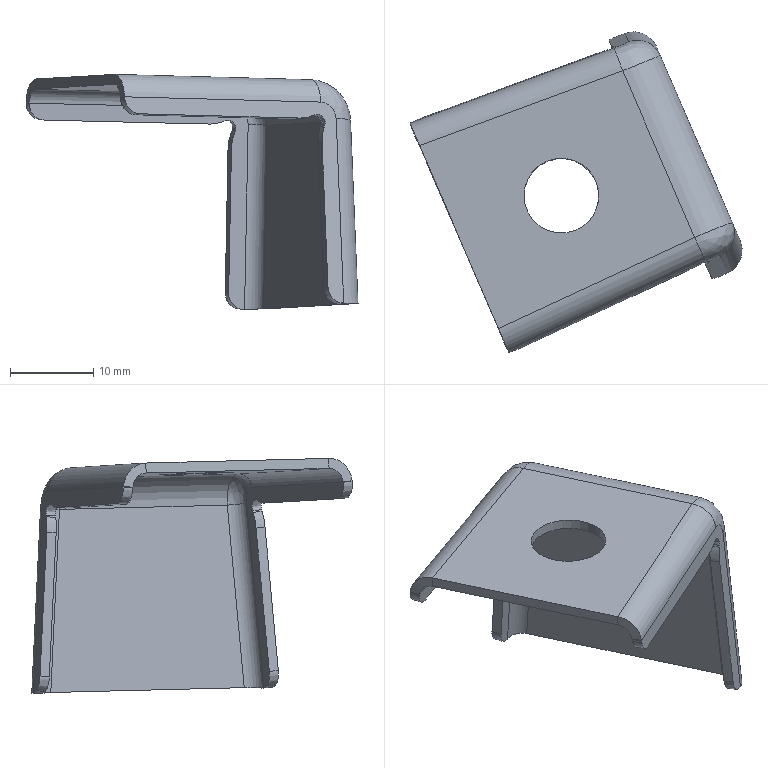Part | 1 solid | 52 faces | box 39.954 x 38.568 x 28.299 mm | volume 2143 mm3 | plane 22 | cylinder 12 | other 10 | spline 8 | commonest cylinder face diameters 3.6 x4 6 x4 9 x2 7.6 x1 10 x1